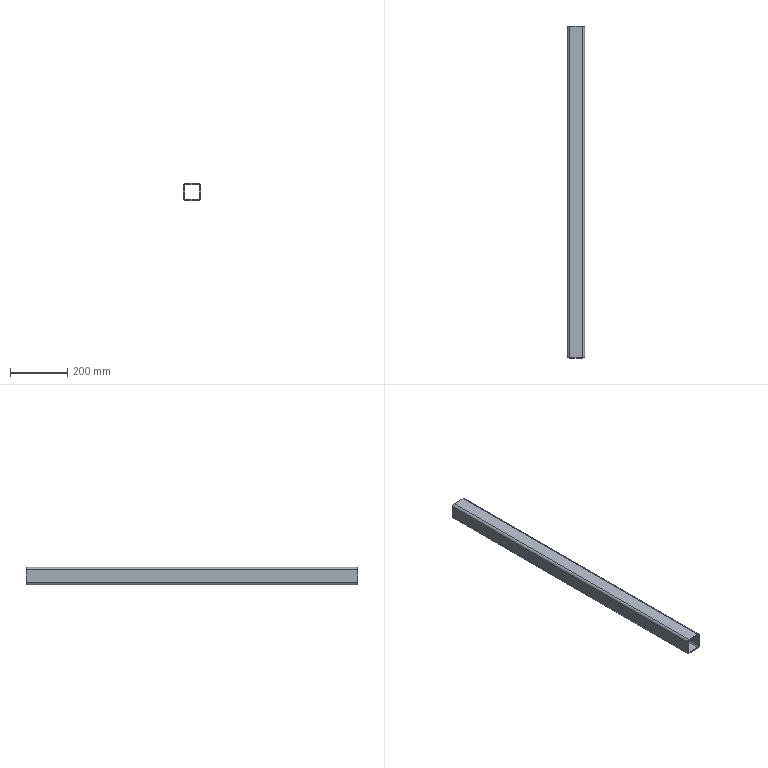Part | SolidWorks | features BaseBody 1 | 1 solid | 18 faces | box 60 x 1160 x 60 mm | volume 991564 mm3 | plane 10 | cylinder 8 | commonest cylinder face diameters 8 x4 16 x4
STEP:
#1=CARTESIAN_POINT('',(-692.,2432.,-1244.));
#2=VERTEX_POINT('',#1);
#3=CARTESIAN_POINT('',(-648.,2432.,-1244.));
#4=VERTEX_POINT('',#3);
#5=CARTESIAN_POINT('',(-648.,2432.,-1244.));
#6=DIRECTION('',(1.,0.,0.));
#7=VECTOR('',#6,1000.);
#8=LINE('',#5,#7);
#9=EDGE_CURVE('',#2,#4,#8,.T.);
#10=ORIENTED_EDGE('',*,*,#9,.T.);
#11=CARTESIAN_POINT('',(-648.,1272.,-1244.));
#12=VERTEX_POINT('',#11);
#13=CARTESIAN_POINT('',(-648.,1242.,-1244.));
#14=DIRECTION('',(0.,-1.,0.));
#15=VECTOR('',#14,1000.);
#16=LINE('',#13,#15);
#17=EDGE_CURVE('',#4,#12,#16,.T.);
#18=ORIENTED_EDGE('',*,*,#17,.T.);
#19=CARTESIAN_POINT('',(-692.,1272.,-1244.));
#20=VERTEX_POINT('',#19);
#21=CARTESIAN_POINT('',(-648.,1272.,-1244.));
#22=DIRECTION('',(-1.,0.,0.));
#23=VECTOR('',#22,1000.);
#24=LINE('',#21,#23);
#25=EDGE_CURVE('',#12,#20,#24,.T.);
#26=ORIENTED_EDGE('',*,*,#25,.T.);
#27=CARTESIAN_POINT('',(-692.,1242.,-1244.));
#28=DIRECTION('',(0.,1.,0.));
#29=VECTOR('',#28,1000.);
#30=LINE('',#27,#29);
#31=EDGE_CURVE('',#20,#2,#30,.T.);
#32=ORIENTED_EDGE('',*,*,#31,.T.);
#33=EDGE_LOOP('',(#10,#18,#26,#32));
#34=FACE_OUTER_BOUND('',#33,.T.);
#35=CARTESIAN_POINT('',(-648.,1242.,-1244.));
#36=DIRECTION('',(0.,0.,-1.));
#37=DIRECTION('',(-1.,0.,0.));
#38=AXIS2_PLACEMENT_3D('',#35,#36,#37);
#39=PLANE('',#38);
#40=ADVANCED_FACE('',(#34),#39,.T.);
#41=ORIENTED_EDGE('',*,*,#17,.F.);
#42=CARTESIAN_POINT('',(-644.,2432.,-1248.));
#43=VERTEX_POINT('',#42);
#44=CARTESIAN_POINT('',(-648.,2432.,-1248.));
#45=DIRECTION('',(0.,-1.,0.));
#46=DIRECTION('',(0.,0.,1.));
#47=AXIS2_PLACEMENT_3D('',#44,#45,#46);
#48=CIRCLE('',#47,4.);
#49=EDGE_CURVE('',#43,#4,#48,.T.);
#50=ORIENTED_EDGE('',*,*,#49,.F.);
#51=CARTESIAN_POINT('',(-644.,1272.,-1248.));
#52=VERTEX_POINT('',#51);
#53=CARTESIAN_POINT('',(-644.,1242.,-1248.));
#54=DIRECTION('',(0.,1.,0.));
#55=VECTOR('',#54,1000.);
#56=LINE('',#53,#55);
#57=EDGE_CURVE('',#52,#43,#56,.T.);
#58=ORIENTED_EDGE('',*,*,#57,.F.);
#59=CARTESIAN_POINT('',(-648.,1272.,-1248.));
#60=DIRECTION('',(0.,1.,0.));
#61=DIRECTION('',(0.,0.,1.));
#62=AXIS2_PLACEMENT_3D('',#59,#60,#61);
#63=CIRCLE('',#62,4.);
#64=EDGE_CURVE('',#12,#52,#63,.T.);
#65=ORIENTED_EDGE('',*,*,#64,.F.);
#66=EDGE_LOOP('',(#41,#50,#58,#65));
#67=FACE_OUTER_BOUND('',#66,.T.);
#68=CARTESIAN_POINT('',(-648.,1242.,-1248.));
#69=DIRECTION('',(0.,1.,0.));
#70=DIRECTION('',(0.,0.,1.));
#71=AXIS2_PLACEMENT_3D('',#68,#69,#70);
#72=CYLINDRICAL_SURFACE('',#71,4.);
#73=ADVANCED_FACE('',(#67),#72,.F.);
#74=CARTESIAN_POINT('',(-696.,2432.,-1248.));
#75=VERTEX_POINT('',#74);
#76=CARTESIAN_POINT('',(-692.,2432.,-1248.));
#77=DIRECTION('',(0.,-1.,0.));
#78=DIRECTION('',(0.,0.,1.));
#79=AXIS2_PLACEMENT_3D('',#76,#77,#78);
#80=CIRCLE('',#79,4.);
#81=EDGE_CURVE('',#2,#75,#80,.T.);
#82=ORIENTED_EDGE('',*,*,#81,.T.);
#83=CARTESIAN_POINT('',(-696.,2432.,-1292.));
#84=VERTEX_POINT('',#83);
#85=CARTESIAN_POINT('',(-696.,2432.,-1270.));
#86=DIRECTION('',(0.,0.,-1.));
#87=VECTOR('',#86,1000.);
#88=LINE('',#85,#87);
#89=EDGE_CURVE('',#75,#84,#88,.T.);
#90=ORIENTED_EDGE('',*,*,#89,.T.);
#91=CARTESIAN_POINT('',(-692.,2432.,-1296.));
#92=VERTEX_POINT('',#91);
#93=CARTESIAN_POINT('',(-692.,2432.,-1292.));
#94=DIRECTION('',(0.,-1.,0.));
#95=DIRECTION('',(0.,0.,1.));
#96=AXIS2_PLACEMENT_3D('',#93,#94,#95);
#97=CIRCLE('',#96,4.);
#98=EDGE_CURVE('',#84,#92,#97,.T.);
#99=ORIENTED_EDGE('',*,*,#98,.T.);
#100=CARTESIAN_POINT('',(-648.,2432.,-1296.));
#101=VERTEX_POINT('',#100);
#102=CARTESIAN_POINT('',(-648.,2432.,-1296.));
#103=DIRECTION('',(1.,0.,0.));
#104=VECTOR('',#103,1000.);
#105=LINE('',#102,#104);
#106=EDGE_CURVE('',#92,#101,#105,.T.);
#107=ORIENTED_EDGE('',*,*,#106,.T.);
#108=CARTESIAN_POINT('',(-644.,2432.,-1292.));
#109=VERTEX_POINT('',#108);
#110=CARTESIAN_POINT('',(-648.,2432.,-1292.));
#111=DIRECTION('',(0.,-1.,0.));
#112=DIRECTION('',(0.,0.,1.));
#113=AXIS2_PLACEMENT_3D('',#110,#111,#112);
#114=CIRCLE('',#113,4.);
#115=EDGE_CURVE('',#101,#109,#114,.T.);
#116=ORIENTED_EDGE('',*,*,#115,.T.);
#117=CARTESIAN_POINT('',(-644.,2432.,-1270.));
#118=DIRECTION('',(0.,0.,1.));
#119=VECTOR('',#118,1000.);
#120=LINE('',#117,#119);
#121=EDGE_CURVE('',#109,#43,#120,.T.);
#122=ORIENTED_EDGE('',*,*,#121,.T.);
#123=ORIENTED_EDGE('',*,*,#49,.T.);
#124=ORIENTED_EDGE('',*,*,#9,.F.);
#125=EDGE_LOOP('',(#82,#90,#99,#107,#116,#122,#123,#124));
#126=FACE_BOUND('',#125,.T.);
#127=CARTESIAN_POINT('',(-692.,2432.,-1240.));
#128=VERTEX_POINT('',#127);
#129=CARTESIAN_POINT('',(-648.,2432.,-1240.));
#130=VERTEX_POINT('',#129);
#131=CARTESIAN_POINT('',(-648.,2432.,-1240.));
#132=DIRECTION('',(1.,0.,0.));
#133=VECTOR('',#132,1000.);
#134=LINE('',#131,#133);
#135=EDGE_CURVE('',#128,#130,#134,.T.);
#136=ORIENTED_EDGE('',*,*,#135,.T.);
#137=CARTESIAN_POINT('',(-640.,2432.,-1248.));
#138=VERTEX_POINT('',#137);
#139=CARTESIAN_POINT('',(-648.,2432.,-1248.));
#140=DIRECTION('',(0.,1.,0.));
#141=DIRECTION('',(0.,0.,1.));
#142=AXIS2_PLACEMENT_3D('',#139,#140,#141);
#143=CIRCLE('',#142,8.);
#144=EDGE_CURVE('',#130,#138,#143,.T.);
#145=ORIENTED_EDGE('',*,*,#144,.T.);
#146=CARTESIAN_POINT('',(-640.,2432.,-1292.));
#147=VERTEX_POINT('',#146);
#148=CARTESIAN_POINT('',(-640.,2432.,-1270.));
#149=DIRECTION('',(0.,0.,-1.));
#150=VECTOR('',#149,1000.);
#151=LINE('',#148,#150);
#152=EDGE_CURVE('',#138,#147,#151,.T.);
#153=ORIENTED_EDGE('',*,*,#152,.T.);
#154=CARTESIAN_POINT('',(-648.,2432.,-1300.));
#155=VERTEX_POINT('',#154);
#156=CARTESIAN_POINT('',(-648.,2432.,-1292.));
#157=DIRECTION('',(0.,1.,0.));
#158=DIRECTION('',(0.,0.,1.));
#159=AXIS2_PLACEMENT_3D('',#156,#157,#158);
#160=CIRCLE('',#159,8.);
#161=EDGE_CURVE('',#147,#155,#160,.T.);
#162=ORIENTED_EDGE('',*,*,#161,.T.);
#163=CARTESIAN_POINT('',(-692.,2432.,-1300.));
#164=VERTEX_POINT('',#163);
#165=CARTESIAN_POINT('',(-648.,2432.,-1300.));
#166=DIRECTION('',(-1.,0.,0.));
#167=VECTOR('',#166,1000.);
#168=LINE('',#165,#167);
#169=EDGE_CURVE('',#155,#164,#168,.T.);
#170=ORIENTED_EDGE('',*,*,#169,.T.);
#171=CARTESIAN_POINT('',(-700.,2432.,-1292.));
#172=VERTEX_POINT('',#171);
#173=CARTESIAN_POINT('',(-692.,2432.,-1292.));
#174=DIRECTION('',(0.,1.,0.));
#175=DIRECTION('',(0.,0.,1.));
#176=AXIS2_PLACEMENT_3D('',#173,#174,#175);
#177=CIRCLE('',#176,8.);
#178=EDGE_CURVE('',#164,#172,#177,.T.);
#179=ORIENTED_EDGE('',*,*,#178,.T.);
#180=CARTESIAN_POINT('',(-700.,2432.,-1248.));
#181=VERTEX_POINT('',#180);
#182=CARTESIAN_POINT('',(-700.,2432.,-1270.));
#183=DIRECTION('',(0.,0.,1.));
#184=VECTOR('',#183,1000.);
#185=LINE('',#182,#184);
#186=EDGE_CURVE('',#172,#181,#185,.T.);
#187=ORIENTED_EDGE('',*,*,#186,.T.);
#188=CARTESIAN_POINT('',(-692.,2432.,-1248.));
#189=DIRECTION('',(0.,1.,0.));
#190=DIRECTION('',(0.,0.,1.));
#191=AXIS2_PLACEMENT_3D('',#188,#189,#190);
#192=CIRCLE('',#191,8.);
#193=EDGE_CURVE('',#181,#128,#192,.T.);
#194=ORIENTED_EDGE('',*,*,#193,.T.);
#195=EDGE_LOOP('',(#136,#145,#153,#162,#170,#179,#187,#194));
#196=FACE_OUTER_BOUND('',#195,.T.);
#197=CARTESIAN_POINT('',(-648.,2432.,-1270.));
#198=DIRECTION('',(0.,1.,0.));
#199=DIRECTION('',(0.,0.,1.));
#200=AXIS2_PLACEMENT_3D('',#197,#198,#199);
#201=PLANE('',#200);
#202=ADVANCED_FACE('',(#126,#196),#201,.T.);
#203=CARTESIAN_POINT('',(-696.,1272.,-1248.));
#204=VERTEX_POINT('',#203);
#205=CARTESIAN_POINT('',(-696.,1242.,-1248.));
#206=DIRECTION('',(0.,-1.,0.));
#207=VECTOR('',#206,1000.);
#208=LINE('',#205,#207);
#209=EDGE_CURVE('',#75,#204,#208,.T.);
#210=ORIENTED_EDGE('',*,*,#209,.F.);
#211=ORIENTED_EDGE('',*,*,#81,.F.);
#212=ORIENTED_EDGE('',*,*,#31,.F.);
#213=CARTESIAN_POINT('',(-692.,1272.,-1248.));
#214=DIRECTION('',(0.,1.,0.));
#215=DIRECTION('',(0.,0.,1.));
#216=AXIS2_PLACEMENT_3D('',#213,#214,#215);
#217=CIRCLE('',#216,4.);
#218=EDGE_CURVE('',#204,#20,#217,.T.);
#219=ORIENTED_EDGE('',*,*,#218,.F.);
#220=EDGE_LOOP('',(#210,#211,#212,#219));
#221=FACE_OUTER_BOUND('',#220,.T.);
#222=CARTESIAN_POINT('',(-692.,1242.,-1248.));
#223=DIRECTION('',(0.,1.,0.));
#224=DIRECTION('',(0.,0.,1.));
#225=AXIS2_PLACEMENT_3D('',#222,#223,#224);
#226=CYLINDRICAL_SURFACE('',#225,4.);
#227=ADVANCED_FACE('',(#221),#226,.F.);
#228=ORIENTED_EDGE('',*,*,#218,.T.);
#229=ORIENTED_EDGE('',*,*,#25,.F.);
#230=ORIENTED_EDGE('',*,*,#64,.T.);
#231=CARTESIAN_POINT('',(-644.,1272.,-1292.));
#232=VERTEX_POINT('',#231);
#233=CARTESIAN_POINT('',(-644.,1272.,530.));
#234=DIRECTION('',(0.,0.,-1.));
#235=VECTOR('',#234,1000.);
#236=LINE('',#233,#235);
#237=EDGE_CURVE('',#52,#232,#236,.T.);
#238=ORIENTED_EDGE('',*,*,#237,.T.);
#239=CARTESIAN_POINT('',(-648.,1272.,-1296.));
#240=VERTEX_POINT('',#239);
#241=CARTESIAN_POINT('',(-648.,1272.,-1292.));
#242=DIRECTION('',(0.,1.,0.));
#243=DIRECTION('',(0.,0.,1.));
#244=AXIS2_PLACEMENT_3D('',#241,#242,#243);
#245=CIRCLE('',#244,4.);
#246=EDGE_CURVE('',#232,#240,#245,.T.);
#247=ORIENTED_EDGE('',*,*,#246,.T.);
#248=CARTESIAN_POINT('',(-692.,1272.,-1296.));
#249=VERTEX_POINT('',#248);
#250=CARTESIAN_POINT('',(-648.,1272.,-1296.));
#251=DIRECTION('',(-1.,0.,0.));
#252=VECTOR('',#251,1000.);
#253=LINE('',#250,#252);
#254=EDGE_CURVE('',#240,#249,#253,.T.);
#255=ORIENTED_EDGE('',*,*,#254,.T.);
#256=CARTESIAN_POINT('',(-696.,1272.,-1292.));
#257=VERTEX_POINT('',#256);
#258=CARTESIAN_POINT('',(-692.,1272.,-1292.));
#259=DIRECTION('',(0.,1.,0.));
#260=DIRECTION('',(0.,0.,1.));
#261=AXIS2_PLACEMENT_3D('',#258,#259,#260);
#262=CIRCLE('',#261,4.);
#263=EDGE_CURVE('',#249,#257,#262,.T.);
#264=ORIENTED_EDGE('',*,*,#263,.T.);
#265=CARTESIAN_POINT('',(-696.,1272.,530.));
#266=DIRECTION('',(0.,0.,1.));
#267=VECTOR('',#266,1000.);
#268=LINE('',#265,#267);
#269=EDGE_CURVE('',#257,#204,#268,.T.);
#270=ORIENTED_EDGE('',*,*,#269,.T.);
#271=EDGE_LOOP('',(#228,#229,#230,#238,#247,#255,#264,#270));
#272=FACE_BOUND('',#271,.T.);
#273=CARTESIAN_POINT('',(-640.,1272.,-1292.));
#274=VERTEX_POINT('',#273);
#275=CARTESIAN_POINT('',(-640.,1272.,-1248.));
#276=VERTEX_POINT('',#275);
#277=CARTESIAN_POINT('',(-640.,1272.,530.));
#278=DIRECTION('',(0.,0.,1.));
#279=VECTOR('',#278,1000.);
#280=LINE('',#277,#279);
#281=EDGE_CURVE('',#274,#276,#280,.T.);
#282=ORIENTED_EDGE('',*,*,#281,.T.);
#283=CARTESIAN_POINT('',(-648.,1272.,-1240.));
#284=VERTEX_POINT('',#283);
#285=CARTESIAN_POINT('',(-648.,1272.,-1248.));
#286=DIRECTION('',(0.,-1.,0.));
#287=DIRECTION('',(0.,0.,1.));
#288=AXIS2_PLACEMENT_3D('',#285,#286,#287);
#289=CIRCLE('',#288,8.);
#290=EDGE_CURVE('',#276,#284,#289,.T.);
#291=ORIENTED_EDGE('',*,*,#290,.T.);
#292=CARTESIAN_POINT('',(-692.,1272.,-1240.));
#293=VERTEX_POINT('',#292);
#294=CARTESIAN_POINT('',(-648.,1272.,-1240.));
#295=DIRECTION('',(-1.,0.,0.));
#296=VECTOR('',#295,1000.);
#297=LINE('',#294,#296);
#298=EDGE_CURVE('',#284,#293,#297,.T.);
#299=ORIENTED_EDGE('',*,*,#298,.T.);
#300=CARTESIAN_POINT('',(-700.,1272.,-1248.));
#301=VERTEX_POINT('',#300);
#302=CARTESIAN_POINT('',(-692.,1272.,-1248.));
#303=DIRECTION('',(0.,-1.,0.));
#304=DIRECTION('',(0.,0.,1.));
#305=AXIS2_PLACEMENT_3D('',#302,#303,#304);
#306=CIRCLE('',#305,8.);
#307=EDGE_CURVE('',#293,#301,#306,.T.);
#308=ORIENTED_EDGE('',*,*,#307,.T.);
#309=CARTESIAN_POINT('',(-700.,1272.,-1292.));
#310=VERTEX_POINT('',#309);
#311=CARTESIAN_POINT('',(-700.,1272.,530.));
#312=DIRECTION('',(0.,0.,-1.));
#313=VECTOR('',#312,1000.);
#314=LINE('',#311,#313);
#315=EDGE_CURVE('',#301,#310,#314,.T.);
#316=ORIENTED_EDGE('',*,*,#315,.T.);
#317=CARTESIAN_POINT('',(-692.,1272.,-1300.));
#318=VERTEX_POINT('',#317);
#319=CARTESIAN_POINT('',(-692.,1272.,-1292.));
#320=DIRECTION('',(0.,-1.,0.));
#321=DIRECTION('',(0.,0.,1.));
#322=AXIS2_PLACEMENT_3D('',#319,#320,#321);
#323=CIRCLE('',#322,8.);
#324=EDGE_CURVE('',#310,#318,#323,.T.);
#325=ORIENTED_EDGE('',*,*,#324,.T.);
#326=CARTESIAN_POINT('',(-648.,1272.,-1300.));
#327=VERTEX_POINT('',#326);
#328=CARTESIAN_POINT('',(-648.,1272.,-1300.));
#329=DIRECTION('',(1.,0.,0.));
#330=VECTOR('',#329,1000.);
#331=LINE('',#328,#330);
#332=EDGE_CURVE('',#318,#327,#331,.T.);
#333=ORIENTED_EDGE('',*,*,#332,.T.);
#334=CARTESIAN_POINT('',(-648.,1272.,-1292.));
#335=DIRECTION('',(0.,-1.,0.));
#336=DIRECTION('',(0.,0.,1.));
#337=AXIS2_PLACEMENT_3D('',#334,#335,#336);
#338=CIRCLE('',#337,8.);
#339=EDGE_CURVE('',#327,#274,#338,.T.);
#340=ORIENTED_EDGE('',*,*,#339,.T.);
#341=EDGE_LOOP('',(#282,#291,#299,#308,#316,#325,#333,#340));
#342=FACE_OUTER_BOUND('',#341,.T.);
#343=CARTESIAN_POINT('',(-648.,1272.,530.));
#344=DIRECTION('',(0.,-1.,0.));
#345=DIRECTION('',(0.,0.,-1.));
#346=AXIS2_PLACEMENT_3D('',#343,#344,#345);
#347=PLANE('',#346);
#348=ADVANCED_FACE('',(#272,#342),#347,.T.);
#349=ORIENTED_EDGE('',*,*,#121,.F.);
#350=CARTESIAN_POINT('',(-644.,1242.,-1292.));
#351=DIRECTION('',(0.,-1.,0.));
#352=VECTOR('',#351,1000.);
#353=LINE('',#350,#352);
#354=EDGE_CURVE('',#109,#232,#353,.T.);
#355=ORIENTED_EDGE('',*,*,#354,.T.);
#356=ORIENTED_EDGE('',*,*,#237,.F.);
#357=ORIENTED_EDGE('',*,*,#57,.T.);
#358=EDGE_LOOP('',(#349,#355,#356,#357));
#359=FACE_OUTER_BOUND('',#358,.T.);
#360=CARTESIAN_POINT('',(-644.,1242.,-1248.));
#361=DIRECTION('',(-1.,0.,0.));
#362=DIRECTION('',(0.,0.,1.));
#363=AXIS2_PLACEMENT_3D('',#360,#361,#362);
#364=PLANE('',#363);
#365=ADVANCED_FACE('',(#359),#364,.T.);
#366=ORIENTED_EDGE('',*,*,#89,.F.);
#367=ORIENTED_EDGE('',*,*,#209,.T.);
#368=ORIENTED_EDGE('',*,*,#269,.F.);
#369=CARTESIAN_POINT('',(-696.,1242.,-1292.));
#370=DIRECTION('',(0.,1.,0.));
#371=VECTOR('',#370,1000.);
#372=LINE('',#369,#371);
#373=EDGE_CURVE('',#257,#84,#372,.T.);
#374=ORIENTED_EDGE('',*,*,#373,.T.);
#375=EDGE_LOOP('',(#366,#367,#368,#374));
#376=FACE_OUTER_BOUND('',#375,.T.);
#377=CARTESIAN_POINT('',(-696.,1242.,-1292.));
#378=DIRECTION('',(1.,0.,0.));
#379=DIRECTION('',(0.,0.,-1.));
#380=AXIS2_PLACEMENT_3D('',#377,#378,#379);
#381=PLANE('',#380);
#382=ADVANCED_FACE('',(#376),#381,.T.);
#383=ORIENTED_EDGE('',*,*,#354,.F.);
#384=ORIENTED_EDGE('',*,*,#115,.F.);
#385=CARTESIAN_POINT('',(-648.,1242.,-1296.));
#386=DIRECTION('',(0.,1.,0.));
#387=VECTOR('',#386,1000.);
#388=LINE('',#385,#387);
#389=EDGE_CURVE('',#240,#101,#388,.T.);
#390=ORIENTED_EDGE('',*,*,#389,.F.);
#391=ORIENTED_EDGE('',*,*,#246,.F.);
#392=EDGE_LOOP('',(#383,#384,#390,#391));
#393=FACE_OUTER_BOUND('',#392,.T.);
#394=CARTESIAN_POINT('',(-648.,1242.,-1292.));
#395=DIRECTION('',(0.,1.,0.));
#396=DIRECTION('',(0.,0.,1.));
#397=AXIS2_PLACEMENT_3D('',#394,#395,#396);
#398=CYLINDRICAL_SURFACE('',#397,4.);
#399=ADVANCED_FACE('',(#393),#398,.F.);
#400=ORIENTED_EDGE('',*,*,#106,.F.);
#401=CARTESIAN_POINT('',(-692.,1242.,-1296.));
#402=DIRECTION('',(0.,-1.,0.));
#403=VECTOR('',#402,1000.);
#404=LINE('',#401,#403);
#405=EDGE_CURVE('',#92,#249,#404,.T.);
#406=ORIENTED_EDGE('',*,*,#405,.T.);
#407=ORIENTED_EDGE('',*,*,#254,.F.);
#408=ORIENTED_EDGE('',*,*,#389,.T.);
#409=EDGE_LOOP('',(#400,#406,#407,#408));
#410=FACE_OUTER_BOUND('',#409,.T.);
#411=CARTESIAN_POINT('',(-692.,1242.,-1296.));
#412=DIRECTION('',(0.,0.,1.));
#413=DIRECTION('',(1.,0.,0.));
#414=AXIS2_PLACEMENT_3D('',#411,#412,#413);
#415=PLANE('',#414);
#416=ADVANCED_FACE('',(#410),#415,.T.);
#417=ORIENTED_EDGE('',*,*,#405,.F.);
#418=ORIENTED_EDGE('',*,*,#98,.F.);
#419=ORIENTED_EDGE('',*,*,#373,.F.);
#420=ORIENTED_EDGE('',*,*,#263,.F.);
#421=EDGE_LOOP('',(#417,#418,#419,#420));
#422=FACE_OUTER_BOUND('',#421,.T.);
#423=CARTESIAN_POINT('',(-692.,1242.,-1292.));
#424=DIRECTION('',(0.,1.,0.));
#425=DIRECTION('',(0.,0.,1.));
#426=AXIS2_PLACEMENT_3D('',#423,#424,#425);
#427=CYLINDRICAL_SURFACE('',#426,4.);
#428=ADVANCED_FACE('',(#422),#427,.F.);
#429=CARTESIAN_POINT('',(-648.,1242.,-1240.));
#430=DIRECTION('',(0.,-1.,0.));
#431=VECTOR('',#430,1000.);
#432=LINE('',#429,#431);
#433=EDGE_CURVE('',#130,#284,#432,.T.);
#434=ORIENTED_EDGE('',*,*,#433,.T.);
#435=ORIENTED_EDGE('',*,*,#290,.F.);
#436=CARTESIAN_POINT('',(-640.,1242.,-1248.));
#437=DIRECTION('',(0.,1.,0.));
#438=VECTOR('',#437,1000.);
#439=LINE('',#436,#438);
#440=EDGE_CURVE('',#276,#138,#439,.T.);
#441=ORIENTED_EDGE('',*,*,#440,.T.);
#442=ORIENTED_EDGE('',*,*,#144,.F.);
#443=EDGE_LOOP('',(#434,#435,#441,#442));
#444=FACE_OUTER_BOUND('',#443,.T.);
#445=CARTESIAN_POINT('',(-648.,1242.,-1248.));
#446=DIRECTION('',(0.,1.,0.));
#447=DIRECTION('',(0.,0.,1.));
#448=AXIS2_PLACEMENT_3D('',#445,#446,#447);
#449=CYLINDRICAL_SURFACE('',#448,8.);
#450=ADVANCED_FACE('',(#444),#449,.T.);
#451=ORIENTED_EDGE('',*,*,#135,.F.);
#452=CARTESIAN_POINT('',(-692.,1242.,-1240.));
#453=DIRECTION('',(0.,1.,0.));
#454=VECTOR('',#453,1000.);
#455=LINE('',#452,#454);
#456=EDGE_CURVE('',#293,#128,#455,.T.);
#457=ORIENTED_EDGE('',*,*,#456,.F.);
#458=ORIENTED_EDGE('',*,*,#298,.F.);
#459=ORIENTED_EDGE('',*,*,#433,.F.);
#460=EDGE_LOOP('',(#451,#457,#458,#459));
#461=FACE_OUTER_BOUND('',#460,.T.);
#462=CARTESIAN_POINT('',(-648.,1242.,-1240.));
#463=DIRECTION('',(0.,0.,-1.));
#464=DIRECTION('',(-1.,0.,0.));
#465=AXIS2_PLACEMENT_3D('',#462,#463,#464);
#466=PLANE('',#465);
#467=ADVANCED_FACE('',(#461),#466,.F.);
#468=CARTESIAN_POINT('',(-700.,1242.,-1248.));
#469=DIRECTION('',(0.,-1.,0.));
#470=VECTOR('',#469,1000.);
#471=LINE('',#468,#470);
#472=EDGE_CURVE('',#181,#301,#471,.T.);
#473=ORIENTED_EDGE('',*,*,#472,.T.);
#474=ORIENTED_EDGE('',*,*,#307,.F.);
#475=ORIENTED_EDGE('',*,*,#456,.T.);
#476=ORIENTED_EDGE('',*,*,#193,.F.);
#477=EDGE_LOOP('',(#473,#474,#475,#476));
#478=FACE_OUTER_BOUND('',#477,.T.);
#479=CARTESIAN_POINT('',(-692.,1242.,-1248.));
#480=DIRECTION('',(0.,1.,0.));
#481=DIRECTION('',(0.,0.,1.));
#482=AXIS2_PLACEMENT_3D('',#479,#480,#481);
#483=CYLINDRICAL_SURFACE('',#482,8.);
#484=ADVANCED_FACE('',(#478),#483,.T.);
#485=ORIENTED_EDGE('',*,*,#186,.F.);
#486=CARTESIAN_POINT('',(-700.,1242.,-1292.));
#487=DIRECTION('',(0.,1.,0.));
#488=VECTOR('',#487,1000.);
#489=LINE('',#486,#488);
#490=EDGE_CURVE('',#310,#172,#489,.T.);
#491=ORIENTED_EDGE('',*,*,#490,.F.);
#492=ORIENTED_EDGE('',*,*,#315,.F.);
#493=ORIENTED_EDGE('',*,*,#472,.F.);
#494=EDGE_LOOP('',(#485,#491,#492,#493));
#495=FACE_OUTER_BOUND('',#494,.T.);
#496=CARTESIAN_POINT('',(-700.,1242.,-1292.));
#497=DIRECTION('',(1.,0.,0.));
#498=DIRECTION('',(0.,0.,-1.));
#499=AXIS2_PLACEMENT_3D('',#496,#497,#498);
#500=PLANE('',#499);
#501=ADVANCED_FACE('',(#495),#500,.F.);
#502=CARTESIAN_POINT('',(-692.,1242.,-1300.));
#503=DIRECTION('',(0.,-1.,0.));
#504=VECTOR('',#503,1000.);
#505=LINE('',#502,#504);
#506=EDGE_CURVE('',#164,#318,#505,.T.);
#507=ORIENTED_EDGE('',*,*,#506,.T.);
#508=ORIENTED_EDGE('',*,*,#324,.F.);
#509=ORIENTED_EDGE('',*,*,#490,.T.);
#510=ORIENTED_EDGE('',*,*,#178,.F.);
#511=EDGE_LOOP('',(#507,#508,#509,#510));
#512=FACE_OUTER_BOUND('',#511,.T.);
#513=CARTESIAN_POINT('',(-692.,1242.,-1292.));
#514=DIRECTION('',(0.,1.,0.));
#515=DIRECTION('',(0.,0.,1.));
#516=AXIS2_PLACEMENT_3D('',#513,#514,#515);
#517=CYLINDRICAL_SURFACE('',#516,8.);
#518=ADVANCED_FACE('',(#512),#517,.T.);
#519=ORIENTED_EDGE('',*,*,#169,.F.);
#520=CARTESIAN_POINT('',(-648.,1242.,-1300.));
#521=DIRECTION('',(0.,1.,0.));
#522=VECTOR('',#521,1000.);
#523=LINE('',#520,#522);
#524=EDGE_CURVE('',#327,#155,#523,.T.);
#525=ORIENTED_EDGE('',*,*,#524,.F.);
#526=ORIENTED_EDGE('',*,*,#332,.F.);
#527=ORIENTED_EDGE('',*,*,#506,.F.);
#528=EDGE_LOOP('',(#519,#525,#526,#527));
#529=FACE_OUTER_BOUND('',#528,.T.);
#530=CARTESIAN_POINT('',(-692.,1242.,-1300.));
#531=DIRECTION('',(0.,0.,1.));
#532=DIRECTION('',(1.,0.,0.));
#533=AXIS2_PLACEMENT_3D('',#530,#531,#532);
#534=PLANE('',#533);
#535=ADVANCED_FACE('',(#529),#534,.F.);
#536=CARTESIAN_POINT('',(-640.,1242.,-1292.));
#537=DIRECTION('',(0.,-1.,0.));
#538=VECTOR('',#537,1000.);
#539=LINE('',#536,#538);
#540=EDGE_CURVE('',#147,#274,#539,.T.);
#541=ORIENTED_EDGE('',*,*,#540,.T.);
#542=ORIENTED_EDGE('',*,*,#339,.F.);
#543=ORIENTED_EDGE('',*,*,#524,.T.);
#544=ORIENTED_EDGE('',*,*,#161,.F.);
#545=EDGE_LOOP('',(#541,#542,#543,#544));
#546=FACE_OUTER_BOUND('',#545,.T.);
#547=CARTESIAN_POINT('',(-648.,1242.,-1292.));
#548=DIRECTION('',(0.,1.,0.));
#549=DIRECTION('',(0.,0.,1.));
#550=AXIS2_PLACEMENT_3D('',#547,#548,#549);
#551=CYLINDRICAL_SURFACE('',#550,8.);
#552=ADVANCED_FACE('',(#546),#551,.T.);
#553=ORIENTED_EDGE('',*,*,#152,.F.);
#554=ORIENTED_EDGE('',*,*,#440,.F.);
#555=ORIENTED_EDGE('',*,*,#281,.F.);
#556=ORIENTED_EDGE('',*,*,#540,.F.);
#557=EDGE_LOOP('',(#553,#554,#555,#556));
#558=FACE_OUTER_BOUND('',#557,.T.);
#559=CARTESIAN_POINT('',(-640.,1242.,-1248.));
#560=DIRECTION('',(-1.,0.,0.));
#561=DIRECTION('',(0.,0.,1.));
#562=AXIS2_PLACEMENT_3D('',#559,#560,#561);
#563=PLANE('',#562);
#564=ADVANCED_FACE('',(#558),#563,.F.);
#565=CLOSED_SHELL('',(#40,#73,#202,#227,#348,#365,#382,#399,#416,#428,#450,#467,#484,#501,#518,#535,#552,#564));
#566=MANIFOLD_SOLID_BREP('',#565);
#567=CARTESIAN_POINT('',(0.,0.,0.));
#568=DIRECTION('',(0.,0.,1.));
#569=DIRECTION('',(1.,0.,0.));
#570=AXIS2_PLACEMENT_3D('',#567,#568,#569);
#571=(LENGTH_UNIT()NAMED_UNIT(*)SI_UNIT(.MILLI.,.METRE.));
#572=UNCERTAINTY_MEASURE_WITH_UNIT(LENGTH_MEASURE(0.00001),#571,'','');
#573=(NAMED_UNIT(*)PLANE_ANGLE_UNIT()SI_UNIT($,.RADIAN.));
#574=(NAMED_UNIT(*)SI_UNIT($,.STERADIAN.)SOLID_ANGLE_UNIT());
#575=(GEOMETRIC_REPRESENTATION_CONTEXT(3)GLOBAL_UNCERTAINTY_ASSIGNED_CONTEXT((#572))GLOBAL_UNIT_ASSIGNED_CONTEXT((#571,#573,#574))REPRESENTATION_CONTEXT('',''));
#576=ADVANCED_BREP_SHAPE_REPRESENTATION('',(#566,#570),#575);